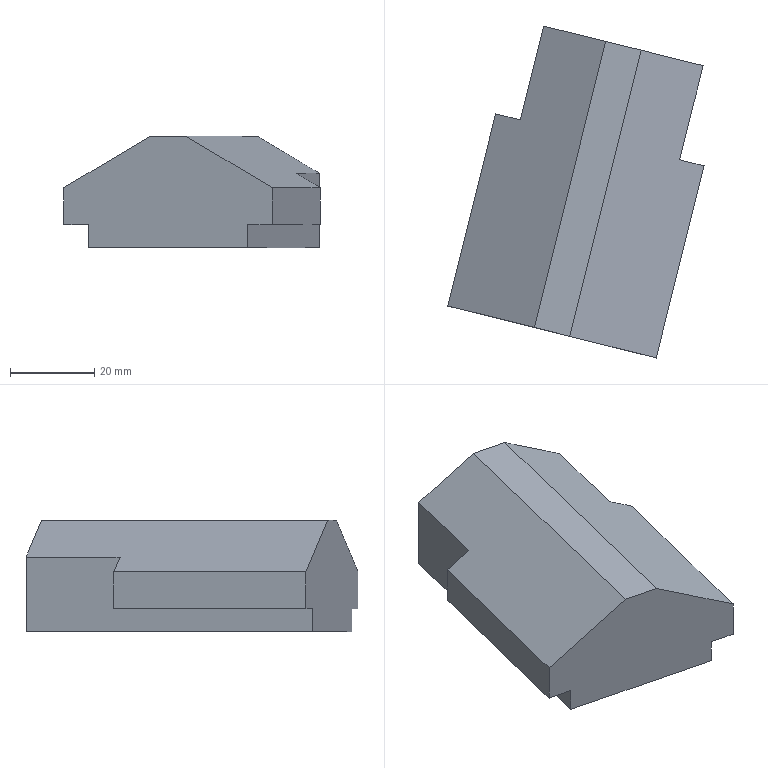Part | NX | features solid 2 | 1 solid | 14 faces | box 60.855 x 78.807 x 26.5 mm | volume 68971 mm3 | plane 14
STEP:
#1=CARTESIAN_POINT('',(-898.093,346.724,23.));
#2=VERTEX_POINT('',#1);
#3=CARTESIAN_POINT('',(-935.934,356.159,23.));
#4=VERTEX_POINT('',#3);
#5=CARTESIAN_POINT('',(-885.479,343.579,23.));
#6=DIRECTION('',(-0.9703,0.2419,0.));
#7=VECTOR('',#6,1000.);
#8=LINE('',#5,#7);
#9=EDGE_CURVE('',#2,#4,#8,.T.);
#10=ORIENTED_EDGE('',*,*,#9,.T.);
#11=CARTESIAN_POINT('',(-919.,424.08,23.));
#12=VERTEX_POINT('',#11);
#13=CARTESIAN_POINT('',(-919.,424.08,23.));
#14=DIRECTION('',(-0.2419,-0.9703,0.));
#15=VECTOR('',#14,1000.);
#16=LINE('',#13,#15);
#17=EDGE_CURVE('',#12,#4,#16,.T.);
#18=ORIENTED_EDGE('',*,*,#17,.F.);
#19=CARTESIAN_POINT('',(-881.158,414.645,23.));
#20=VERTEX_POINT('',#19);
#21=CARTESIAN_POINT('',(-868.545,411.5,23.));
#22=DIRECTION('',(-0.9703,0.2419,0.));
#23=VECTOR('',#22,1000.);
#24=LINE('',#21,#23);
#25=EDGE_CURVE('',#20,#12,#24,.T.);
#26=ORIENTED_EDGE('',*,*,#25,.F.);
#27=CARTESIAN_POINT('',(-881.158,414.645,23.));
#28=DIRECTION('',(-0.2419,-0.9703,0.));
#29=VECTOR('',#28,1000.);
#30=LINE('',#27,#29);
#31=EDGE_CURVE('',#20,#2,#30,.T.);
#32=ORIENTED_EDGE('',*,*,#31,.T.);
#33=EDGE_LOOP('',(#10,#18,#26,#32));
#34=FACE_BOUND('',#33,.T.);
#35=CARTESIAN_POINT('',(-891.527,319.321,23.));
#36=DIRECTION('',(0.,0.,-1.));
#37=DIRECTION('',(-0.9703,0.2419,0.));
#38=AXIS2_PLACEMENT_3D('',#35,#36,#37);
#39=PLANE('',#38);
#40=ADVANCED_FACE('',(#34),#39,.T.);
#41=CARTESIAN_POINT('',(-924.564,401.763,40.741));
#42=VERTEX_POINT('',#41);
#43=CARTESIAN_POINT('',(-924.564,401.763,28.5));
#44=VERTEX_POINT('',#43);
#45=CARTESIAN_POINT('',(-924.564,401.763,40.741));
#46=DIRECTION('',(0.,0.,-1.));
#47=VECTOR('',#46,1000.);
#48=LINE('',#45,#47);
#49=EDGE_CURVE('',#42,#44,#48,.T.);
#50=ORIENTED_EDGE('',*,*,#49,.F.);
#51=CARTESIAN_POINT('',(-919.,424.08,40.741));
#52=VERTEX_POINT('',#51);
#53=CARTESIAN_POINT('',(-919.,424.08,40.741));
#54=DIRECTION('',(-0.2419,-0.9703,0.));
#55=VECTOR('',#54,1000.);
#56=LINE('',#53,#55);
#57=EDGE_CURVE('',#52,#42,#56,.T.);
#58=ORIENTED_EDGE('',*,*,#57,.F.);
#59=CARTESIAN_POINT('',(-919.,424.08,40.741));
#60=DIRECTION('',(0.,0.,-1.));
#61=VECTOR('',#60,1000.);
#62=LINE('',#59,#61);
#63=EDGE_CURVE('',#52,#12,#62,.T.);
#64=ORIENTED_EDGE('',*,*,#63,.T.);
#65=ORIENTED_EDGE('',*,*,#17,.T.);
#66=CARTESIAN_POINT('',(-935.934,356.159,28.5));
#67=VERTEX_POINT('',#66);
#68=CARTESIAN_POINT('',(-935.934,356.159,40.741));
#69=DIRECTION('',(0.,0.,-1.));
#70=VECTOR('',#69,1000.);
#71=LINE('',#68,#70);
#72=EDGE_CURVE('',#67,#4,#71,.T.);
#73=ORIENTED_EDGE('',*,*,#72,.F.);
#74=CARTESIAN_POINT('',(-919.,424.08,28.5));
#75=DIRECTION('',(-0.2419,-0.9703,0.));
#76=VECTOR('',#75,1000.);
#77=LINE('',#74,#76);
#78=EDGE_CURVE('',#44,#67,#77,.T.);
#79=ORIENTED_EDGE('',*,*,#78,.F.);
#80=EDGE_LOOP('',(#50,#58,#64,#65,#73,#79));
#81=FACE_BOUND('',#80,.T.);
#82=CARTESIAN_POINT('',(-919.,424.08,40.741));
#83=DIRECTION('',(0.9703,-0.2419,0.));
#84=DIRECTION('',(-0.1022,-0.4101,-0.9063));
#85=AXIS2_PLACEMENT_3D('',#82,#83,#84);
#86=PLANE('',#85);
#87=ADVANCED_FACE('',(#81),#86,.F.);
#88=CARTESIAN_POINT('',(-921.215,352.489,49.5));
#89=VERTEX_POINT('',#88);
#90=CARTESIAN_POINT('',(-941.756,357.61,37.277));
#91=VERTEX_POINT('',#90);
#92=CARTESIAN_POINT('',(-921.865,352.651,49.113));
#93=DIRECTION('',(-0.8403,0.2095,-0.5));
#94=VECTOR('',#93,1000.);
#95=LINE('',#92,#94);
#96=EDGE_CURVE('',#89,#91,#95,.T.);
#97=ORIENTED_EDGE('',*,*,#96,.F.);
#98=CARTESIAN_POINT('',(-904.28,420.409,49.5));
#99=VERTEX_POINT('',#98);
#100=CARTESIAN_POINT('',(-904.28,420.409,49.5));
#101=DIRECTION('',(-0.2419,-0.9703,0.));
#102=VECTOR('',#101,1000.);
#103=LINE('',#100,#102);
#104=EDGE_CURVE('',#99,#89,#103,.T.);
#105=ORIENTED_EDGE('',*,*,#104,.F.);
#106=CARTESIAN_POINT('',(-904.931,420.572,49.113));
#107=DIRECTION('',(-0.8403,0.2095,-0.5));
#108=VECTOR('',#107,1000.);
#109=LINE('',#106,#108);
#110=EDGE_CURVE('',#99,#52,#109,.T.);
#111=ORIENTED_EDGE('',*,*,#110,.T.);
#112=ORIENTED_EDGE('',*,*,#57,.T.);
#113=CARTESIAN_POINT('',(-930.386,403.214,37.277));
#114=VERTEX_POINT('',#113);
#115=CARTESIAN_POINT('',(-930.386,403.214,37.277));
#116=DIRECTION('',(0.8403,-0.2095,0.5));
#117=VECTOR('',#116,1000.);
#118=LINE('',#115,#117);
#119=EDGE_CURVE('',#114,#42,#118,.T.);
#120=ORIENTED_EDGE('',*,*,#119,.F.);
#121=CARTESIAN_POINT('',(-930.386,403.214,37.277));
#122=DIRECTION('',(-0.2419,-0.9703,0.));
#123=VECTOR('',#122,1000.);
#124=LINE('',#121,#123);
#125=EDGE_CURVE('',#114,#91,#124,.T.);
#126=ORIENTED_EDGE('',*,*,#125,.T.);
#127=EDGE_LOOP('',(#97,#105,#111,#112,#120,#126));
#128=FACE_BOUND('',#127,.T.);
#129=CARTESIAN_POINT('',(-904.931,420.572,49.113));
#130=DIRECTION('',(0.4851,-0.121,-0.866));
#131=DIRECTION('',(-0.8733,-0.01628,-0.4869));
#132=AXIS2_PLACEMENT_3D('',#129,#130,#131);
#133=PLANE('',#132);
#134=ADVANCED_FACE('',(#128),#133,.F.);
#135=CARTESIAN_POINT('',(-912.813,350.394,49.5));
#136=VERTEX_POINT('',#135);
#137=CARTESIAN_POINT('',(-912.162,350.232,49.5));
#138=DIRECTION('',(-0.9703,0.2419,0.));
#139=VECTOR('',#138,1000.);
#140=LINE('',#137,#139);
#141=EDGE_CURVE('',#136,#89,#140,.T.);
#142=ORIENTED_EDGE('',*,*,#141,.F.);
#143=CARTESIAN_POINT('',(-895.878,418.315,49.5));
#144=VERTEX_POINT('',#143);
#145=CARTESIAN_POINT('',(-895.878,418.315,49.5));
#146=DIRECTION('',(-0.2419,-0.9703,0.));
#147=VECTOR('',#146,1000.);
#148=LINE('',#145,#147);
#149=EDGE_CURVE('',#144,#136,#148,.T.);
#150=ORIENTED_EDGE('',*,*,#149,.F.);
#151=CARTESIAN_POINT('',(-895.228,418.152,49.5));
#152=DIRECTION('',(-0.9703,0.2419,0.));
#153=VECTOR('',#152,1000.);
#154=LINE('',#151,#153);
#155=EDGE_CURVE('',#144,#99,#154,.T.);
#156=ORIENTED_EDGE('',*,*,#155,.T.);
#157=ORIENTED_EDGE('',*,*,#104,.T.);
#158=EDGE_LOOP('',(#142,#150,#156,#157));
#159=FACE_BOUND('',#158,.T.);
#160=CARTESIAN_POINT('',(-895.228,418.152,49.5));
#161=DIRECTION('',(0.,0.,-1.));
#162=DIRECTION('',(-0.2419,-0.9703,0.));
#163=AXIS2_PLACEMENT_3D('',#160,#161,#162);
#164=PLANE('',#163);
#165=ADVANCED_FACE('',(#159),#164,.F.);
#166=CARTESIAN_POINT('',(-892.271,345.272,37.277));
#167=VERTEX_POINT('',#166);
#168=CARTESIAN_POINT('',(-898.093,346.724,40.741));
#169=DIRECTION('',(-0.8403,0.2095,0.5));
#170=VECTOR('',#169,1000.);
#171=LINE('',#168,#170);
#172=EDGE_CURVE('',#167,#136,#171,.T.);
#173=ORIENTED_EDGE('',*,*,#172,.F.);
#174=CARTESIAN_POINT('',(-880.901,390.876,37.277));
#175=VERTEX_POINT('',#174);
#176=CARTESIAN_POINT('',(-880.901,390.876,37.277));
#177=DIRECTION('',(-0.2419,-0.9703,0.));
#178=VECTOR('',#177,1000.);
#179=LINE('',#176,#178);
#180=EDGE_CURVE('',#175,#167,#179,.T.);
#181=ORIENTED_EDGE('',*,*,#180,.F.);
#182=CARTESIAN_POINT('',(-886.723,392.328,40.741));
#183=VERTEX_POINT('',#182);
#184=CARTESIAN_POINT('',(-880.901,390.876,37.277));
#185=DIRECTION('',(-0.8403,0.2095,0.5));
#186=VECTOR('',#185,1000.);
#187=LINE('',#184,#186);
#188=EDGE_CURVE('',#175,#183,#187,.T.);
#189=ORIENTED_EDGE('',*,*,#188,.T.);
#190=CARTESIAN_POINT('',(-881.158,414.645,40.741));
#191=VERTEX_POINT('',#190);
#192=CARTESIAN_POINT('',(-881.158,414.645,40.741));
#193=DIRECTION('',(-0.2419,-0.9703,0.));
#194=VECTOR('',#193,1000.);
#195=LINE('',#192,#194);
#196=EDGE_CURVE('',#191,#183,#195,.T.);
#197=ORIENTED_EDGE('',*,*,#196,.F.);
#198=CARTESIAN_POINT('',(-881.158,414.645,40.741));
#199=DIRECTION('',(-0.8403,0.2095,0.5));
#200=VECTOR('',#199,1000.);
#201=LINE('',#198,#200);
#202=EDGE_CURVE('',#191,#144,#201,.T.);
#203=ORIENTED_EDGE('',*,*,#202,.T.);
#204=ORIENTED_EDGE('',*,*,#149,.T.);
#205=EDGE_LOOP('',(#173,#181,#189,#197,#203,#204));
#206=FACE_BOUND('',#205,.T.);
#207=CARTESIAN_POINT('',(-881.158,414.645,40.741));
#208=DIRECTION('',(-0.4851,0.121,-0.866));
#209=DIRECTION('',(-0.7634,0.4244,0.4869));
#210=AXIS2_PLACEMENT_3D('',#207,#208,#209);
#211=PLANE('',#210);
#212=ADVANCED_FACE('',(#206),#211,.F.);
#213=CARTESIAN_POINT('',(-886.723,392.328,28.5));
#214=VERTEX_POINT('',#213);
#215=CARTESIAN_POINT('',(-898.093,346.724,28.5));
#216=VERTEX_POINT('',#215);
#217=CARTESIAN_POINT('',(-881.158,414.645,28.5));
#218=DIRECTION('',(-0.2419,-0.9703,0.));
#219=VECTOR('',#218,1000.);
#220=LINE('',#217,#219);
#221=EDGE_CURVE('',#214,#216,#220,.T.);
#222=ORIENTED_EDGE('',*,*,#221,.T.);
#223=CARTESIAN_POINT('',(-898.093,346.724,40.741));
#224=DIRECTION('',(0.,0.,-1.));
#225=VECTOR('',#224,1000.);
#226=LINE('',#223,#225);
#227=EDGE_CURVE('',#216,#2,#226,.T.);
#228=ORIENTED_EDGE('',*,*,#227,.T.);
#229=ORIENTED_EDGE('',*,*,#31,.F.);
#230=CARTESIAN_POINT('',(-881.158,414.645,40.741));
#231=DIRECTION('',(0.,0.,-1.));
#232=VECTOR('',#231,1000.);
#233=LINE('',#230,#232);
#234=EDGE_CURVE('',#191,#20,#233,.T.);
#235=ORIENTED_EDGE('',*,*,#234,.F.);
#236=ORIENTED_EDGE('',*,*,#196,.T.);
#237=CARTESIAN_POINT('',(-886.723,392.328,40.741));
#238=DIRECTION('',(0.,0.,-1.));
#239=VECTOR('',#238,1000.);
#240=LINE('',#237,#239);
#241=EDGE_CURVE('',#183,#214,#240,.T.);
#242=ORIENTED_EDGE('',*,*,#241,.T.);
#243=EDGE_LOOP('',(#222,#228,#229,#235,#236,#242));
#244=FACE_BOUND('',#243,.T.);
#245=CARTESIAN_POINT('',(-881.158,414.645,40.741));
#246=DIRECTION('',(0.9703,-0.2419,0.));
#247=DIRECTION('',(-0.2193,-0.8794,0.4226));
#248=AXIS2_PLACEMENT_3D('',#245,#246,#247);
#249=PLANE('',#248);
#250=ADVANCED_FACE('',(#244),#249,.T.);
#251=ORIENTED_EDGE('',*,*,#25,.T.);
#252=ORIENTED_EDGE('',*,*,#63,.F.);
#253=ORIENTED_EDGE('',*,*,#110,.F.);
#254=ORIENTED_EDGE('',*,*,#155,.F.);
#255=ORIENTED_EDGE('',*,*,#202,.F.);
#256=ORIENTED_EDGE('',*,*,#234,.T.);
#257=EDGE_LOOP('',(#251,#252,#253,#254,#255,#256));
#258=FACE_BOUND('',#257,.T.);
#259=CARTESIAN_POINT('',(-881.158,414.645,19.5));
#260=DIRECTION('',(0.2419,0.9703,0.));
#261=DIRECTION('',(0.,0.,-1.));
#262=AXIS2_PLACEMENT_3D('',#259,#260,#261);
#263=PLANE('',#262);
#264=ADVANCED_FACE('',(#258),#263,.T.);
#265=ORIENTED_EDGE('',*,*,#9,.F.);
#266=ORIENTED_EDGE('',*,*,#227,.F.);
#267=CARTESIAN_POINT('',(-892.271,345.272,28.5));
#268=VERTEX_POINT('',#267);
#269=CARTESIAN_POINT('',(-892.271,345.272,28.5));
#270=DIRECTION('',(-0.9703,0.2419,0.));
#271=VECTOR('',#270,1000.);
#272=LINE('',#269,#271);
#273=EDGE_CURVE('',#268,#216,#272,.T.);
#274=ORIENTED_EDGE('',*,*,#273,.F.);
#275=CARTESIAN_POINT('',(-892.271,345.272,37.277));
#276=DIRECTION('',(0.,0.,-1.));
#277=VECTOR('',#276,1000.);
#278=LINE('',#275,#277);
#279=EDGE_CURVE('',#167,#268,#278,.T.);
#280=ORIENTED_EDGE('',*,*,#279,.F.);
#281=ORIENTED_EDGE('',*,*,#172,.T.);
#282=ORIENTED_EDGE('',*,*,#141,.T.);
#283=ORIENTED_EDGE('',*,*,#96,.T.);
#284=CARTESIAN_POINT('',(-941.756,357.61,28.5));
#285=VERTEX_POINT('',#284);
#286=CARTESIAN_POINT('',(-941.756,357.61,37.277));
#287=DIRECTION('',(0.,0.,-1.));
#288=VECTOR('',#287,1000.);
#289=LINE('',#286,#288);
#290=EDGE_CURVE('',#91,#285,#289,.T.);
#291=ORIENTED_EDGE('',*,*,#290,.T.);
#292=CARTESIAN_POINT('',(-941.756,357.61,28.5));
#293=DIRECTION('',(0.9703,-0.2419,0.));
#294=VECTOR('',#293,1000.);
#295=LINE('',#292,#294);
#296=EDGE_CURVE('',#285,#67,#295,.T.);
#297=ORIENTED_EDGE('',*,*,#296,.T.);
#298=ORIENTED_EDGE('',*,*,#72,.T.);
#299=EDGE_LOOP('',(#265,#266,#274,#280,#281,#282,#283,#291,#297,#298));
#300=FACE_BOUND('',#299,.T.);
#301=CARTESIAN_POINT('',(-898.093,346.724,19.5));
#302=DIRECTION('',(0.2419,0.9703,0.));
#303=DIRECTION('',(0.,0.,-1.));
#304=AXIS2_PLACEMENT_3D('',#301,#302,#303);
#305=PLANE('',#304);
#306=ADVANCED_FACE('',(#300),#305,.F.);
#307=CARTESIAN_POINT('',(-880.901,390.876,28.5));
#308=VERTEX_POINT('',#307);
#309=CARTESIAN_POINT('',(-880.901,390.876,37.277));
#310=DIRECTION('',(0.,0.,-1.));
#311=VECTOR('',#310,1000.);
#312=LINE('',#309,#311);
#313=EDGE_CURVE('',#175,#308,#312,.T.);
#314=ORIENTED_EDGE('',*,*,#313,.F.);
#315=ORIENTED_EDGE('',*,*,#180,.T.);
#316=ORIENTED_EDGE('',*,*,#279,.T.);
#317=CARTESIAN_POINT('',(-875.337,413.193,28.5));
#318=DIRECTION('',(-0.2419,-0.9703,0.));
#319=VECTOR('',#318,1000.);
#320=LINE('',#317,#319);
#321=EDGE_CURVE('',#308,#268,#320,.T.);
#322=ORIENTED_EDGE('',*,*,#321,.F.);
#323=EDGE_LOOP('',(#314,#315,#316,#322));
#324=FACE_BOUND('',#323,.T.);
#325=CARTESIAN_POINT('',(-880.901,390.876,37.277));
#326=DIRECTION('',(0.9703,-0.2419,0.));
#327=DIRECTION('',(-0.1022,-0.4101,-0.9063));
#328=AXIS2_PLACEMENT_3D('',#325,#326,#327);
#329=PLANE('',#328);
#330=ADVANCED_FACE('',(#324),#329,.T.);
#331=ORIENTED_EDGE('',*,*,#241,.F.);
#332=ORIENTED_EDGE('',*,*,#188,.F.);
#333=ORIENTED_EDGE('',*,*,#313,.T.);
#334=CARTESIAN_POINT('',(-886.723,392.328,28.5));
#335=DIRECTION('',(0.9703,-0.2419,0.));
#336=VECTOR('',#335,1000.);
#337=LINE('',#334,#336);
#338=EDGE_CURVE('',#214,#308,#337,.T.);
#339=ORIENTED_EDGE('',*,*,#338,.F.);
#340=EDGE_LOOP('',(#331,#332,#333,#339));
#341=FACE_BOUND('',#340,.T.);
#342=CARTESIAN_POINT('',(-886.723,392.328,19.5));
#343=DIRECTION('',(0.2419,0.9703,0.));
#344=DIRECTION('',(0.,0.,-1.));
#345=AXIS2_PLACEMENT_3D('',#342,#343,#344);
#346=PLANE('',#345);
#347=ADVANCED_FACE('',(#341),#346,.T.);
#348=ORIENTED_EDGE('',*,*,#221,.F.);
#349=ORIENTED_EDGE('',*,*,#338,.T.);
#350=ORIENTED_EDGE('',*,*,#321,.T.);
#351=ORIENTED_EDGE('',*,*,#273,.T.);
#352=EDGE_LOOP('',(#348,#349,#350,#351));
#353=FACE_BOUND('',#352,.T.);
#354=CARTESIAN_POINT('',(-875.337,413.193,28.5));
#355=DIRECTION('',(0.,0.,-1.));
#356=DIRECTION('',(-0.2419,-0.9703,0.));
#357=AXIS2_PLACEMENT_3D('',#354,#355,#356);
#358=PLANE('',#357);
#359=ADVANCED_FACE('',(#353),#358,.T.);
#360=CARTESIAN_POINT('',(-930.386,403.214,28.5));
#361=VERTEX_POINT('',#360);
#362=CARTESIAN_POINT('',(-930.386,403.214,37.277));
#363=DIRECTION('',(0.,0.,-1.));
#364=VECTOR('',#363,1000.);
#365=LINE('',#362,#364);
#366=EDGE_CURVE('',#114,#361,#365,.T.);
#367=ORIENTED_EDGE('',*,*,#366,.T.);
#368=CARTESIAN_POINT('',(-924.822,425.531,28.5));
#369=DIRECTION('',(-0.2419,-0.9703,0.));
#370=VECTOR('',#369,1000.);
#371=LINE('',#368,#370);
#372=EDGE_CURVE('',#361,#285,#371,.T.);
#373=ORIENTED_EDGE('',*,*,#372,.T.);
#374=ORIENTED_EDGE('',*,*,#290,.F.);
#375=ORIENTED_EDGE('',*,*,#125,.F.);
#376=EDGE_LOOP('',(#367,#373,#374,#375));
#377=FACE_BOUND('',#376,.T.);
#378=CARTESIAN_POINT('',(-930.386,403.214,37.277));
#379=DIRECTION('',(-0.9703,0.2419,0.));
#380=DIRECTION('',(-0.1022,-0.4101,-0.9063));
#381=AXIS2_PLACEMENT_3D('',#378,#379,#380);
#382=PLANE('',#381);
#383=ADVANCED_FACE('',(#377),#382,.T.);
#384=ORIENTED_EDGE('',*,*,#49,.T.);
#385=CARTESIAN_POINT('',(-924.564,401.763,28.5));
#386=DIRECTION('',(-0.9703,0.2419,0.));
#387=VECTOR('',#386,1000.);
#388=LINE('',#385,#387);
#389=EDGE_CURVE('',#44,#361,#388,.T.);
#390=ORIENTED_EDGE('',*,*,#389,.T.);
#391=ORIENTED_EDGE('',*,*,#366,.F.);
#392=ORIENTED_EDGE('',*,*,#119,.T.);
#393=EDGE_LOOP('',(#384,#390,#391,#392));
#394=FACE_BOUND('',#393,.T.);
#395=CARTESIAN_POINT('',(-924.564,401.763,19.5));
#396=DIRECTION('',(0.2419,0.9703,0.));
#397=DIRECTION('',(0.,0.,-1.));
#398=AXIS2_PLACEMENT_3D('',#395,#396,#397);
#399=PLANE('',#398);
#400=ADVANCED_FACE('',(#394),#399,.T.);
#401=ORIENTED_EDGE('',*,*,#78,.T.);
#402=ORIENTED_EDGE('',*,*,#296,.F.);
#403=ORIENTED_EDGE('',*,*,#372,.F.);
#404=ORIENTED_EDGE('',*,*,#389,.F.);
#405=EDGE_LOOP('',(#401,#402,#403,#404));
#406=FACE_BOUND('',#405,.T.);
#407=CARTESIAN_POINT('',(-924.822,425.531,28.5));
#408=DIRECTION('',(0.,0.,-1.));
#409=DIRECTION('',(-0.2419,-0.9703,0.));
#410=AXIS2_PLACEMENT_3D('',#407,#408,#409);
#411=PLANE('',#410);
#412=ADVANCED_FACE('',(#406),#411,.T.);
#413=CLOSED_SHELL('',(#40,#87,#134,#165,#212,#250,#264,#306,#330,#347,#359,#383,#400,#412));
#414=MANIFOLD_SOLID_BREP('',#413);
#415=(LENGTH_UNIT()NAMED_UNIT(*)SI_UNIT(.MILLI.,.METRE.));
#416=UNCERTAINTY_MEASURE_WITH_UNIT(LENGTH_MEASURE(0.00001),#415,'','');
#417=(NAMED_UNIT(*)PLANE_ANGLE_UNIT()SI_UNIT($,.RADIAN.));
#418=(NAMED_UNIT(*)SI_UNIT($,.STERADIAN.)SOLID_ANGLE_UNIT());
#419=(GEOMETRIC_REPRESENTATION_CONTEXT(3)GLOBAL_UNCERTAINTY_ASSIGNED_CONTEXT((#416))GLOBAL_UNIT_ASSIGNED_CONTEXT((#415,#417,#418))REPRESENTATION_CONTEXT('',''));
#420=ADVANCED_BREP_SHAPE_REPRESENTATION('',(#414),#419);